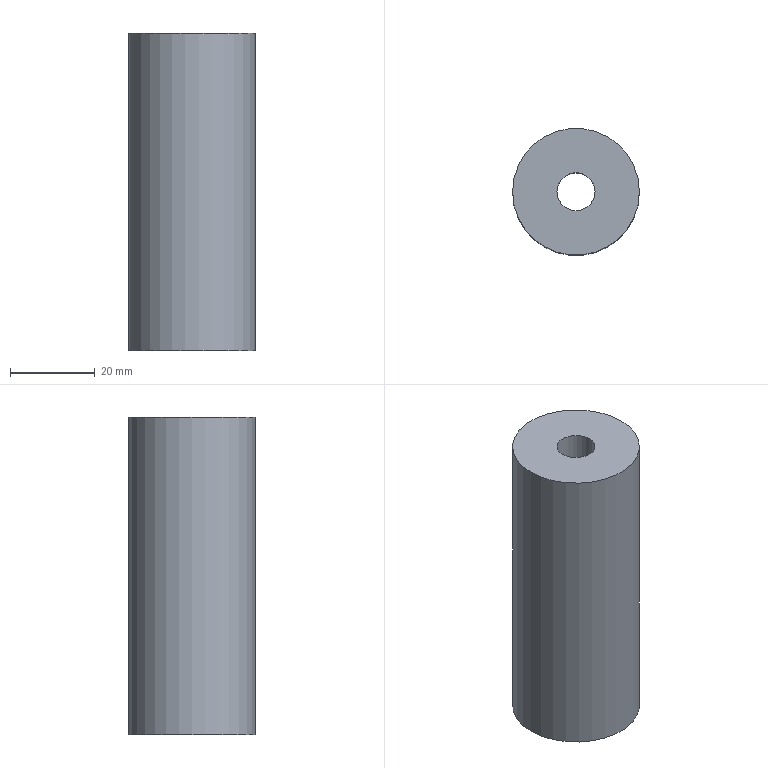Part | NX | features solid 2 | 1 solid | 6 faces | box 30 x 30 x 75 mm | volume 44179 mm3 | cylinder 3 | plane 3 | commonest cylinder face diameters 9 x1 14 x1 30 x1
STEP:
#1=CARTESIAN_POINT('',(-350.023,88.529,-15.002));
#2=VERTEX_POINT('',#1);
#3=CARTESIAN_POINT('',(-335.023,88.529,-15.002));
#4=DIRECTION('',(-0.000000053,0.000000517,-1.));
#5=DIRECTION('',(-1.,0.,0.000000053));
#6=AXIS2_PLACEMENT_3D('',#3,#4,#5);
#7=CIRCLE('',#6,15.);
#8=EDGE_CURVE('',#2,#2,#7,.T.);
#9=ORIENTED_EDGE('',*,*,#8,.F.);
#10=EDGE_LOOP('',(#9));
#11=FACE_BOUND('',#10,.T.);
#12=CARTESIAN_POINT('',(-320.023,88.529,59.998));
#13=VERTEX_POINT('',#12);
#14=CARTESIAN_POINT('',(-335.023,88.529,59.998));
#15=DIRECTION('',(0.000000053,-0.000000517,1.));
#16=DIRECTION('',(1.,0.,-0.000000053));
#17=AXIS2_PLACEMENT_3D('',#14,#15,#16);
#18=CIRCLE('',#17,15.);
#19=EDGE_CURVE('',#13,#13,#18,.F.);
#20=ORIENTED_EDGE('',*,*,#19,.T.);
#21=EDGE_LOOP('',(#20));
#22=FACE_BOUND('',#21,.T.);
#23=CARTESIAN_POINT('',(-335.023,88.529,-24.));
#24=DIRECTION('',(-0.000000053,0.000000517,-1.));
#25=DIRECTION('',(0.,-1.,-0.000000517));
#26=AXIS2_PLACEMENT_3D('',#23,#24,#25);
#27=CYLINDRICAL_SURFACE('',#26,15.);
#28=ADVANCED_FACE('',(#11,#22),#27,.T.);
#29=CARTESIAN_POINT('',(-339.523,88.529,59.998));
#30=VERTEX_POINT('',#29);
#31=CARTESIAN_POINT('',(-335.023,88.529,59.998));
#32=DIRECTION('',(0.000000053,-0.000000517,1.));
#33=DIRECTION('',(-1.,0.,0.000000053));
#34=AXIS2_PLACEMENT_3D('',#31,#32,#33);
#35=CIRCLE('',#34,4.5);
#36=EDGE_CURVE('',#30,#30,#35,.T.);
#37=ORIENTED_EDGE('',*,*,#36,.T.);
#38=EDGE_LOOP('',(#37));
#39=FACE_BOUND('',#38,.T.);
#40=CARTESIAN_POINT('',(-339.523,88.529,29.998));
#41=VERTEX_POINT('',#40);
#42=CARTESIAN_POINT('',(-335.023,88.529,29.998));
#43=DIRECTION('',(0.000000053,-0.000000517,1.));
#44=DIRECTION('',(-1.,0.,0.000000053));
#45=AXIS2_PLACEMENT_3D('',#42,#43,#44);
#46=CIRCLE('',#45,4.5);
#47=EDGE_CURVE('',#41,#41,#46,.T.);
#48=ORIENTED_EDGE('',*,*,#47,.F.);
#49=EDGE_LOOP('',(#48));
#50=FACE_BOUND('',#49,.T.);
#51=CARTESIAN_POINT('',(-335.023,88.529,-64.));
#52=DIRECTION('',(0.000000053,-0.000000517,1.));
#53=DIRECTION('',(0.,-1.,-0.000000517));
#54=AXIS2_PLACEMENT_3D('',#51,#52,#53);
#55=CYLINDRICAL_SURFACE('',#54,4.5);
#56=ADVANCED_FACE('',(#39,#50),#55,.F.);
#57=ORIENTED_EDGE('',*,*,#47,.T.);
#58=EDGE_LOOP('',(#57));
#59=FACE_BOUND('',#58,.T.);
#60=CARTESIAN_POINT('',(-342.023,88.529,29.998));
#61=VERTEX_POINT('',#60);
#62=CARTESIAN_POINT('',(-335.023,88.529,29.998));
#63=DIRECTION('',(0.000000053,-0.000000517,1.));
#64=DIRECTION('',(-1.,0.,0.000000053));
#65=AXIS2_PLACEMENT_3D('',#62,#63,#64);
#66=CIRCLE('',#65,7.);
#67=EDGE_CURVE('',#61,#61,#66,.T.);
#68=ORIENTED_EDGE('',*,*,#67,.F.);
#69=EDGE_LOOP('',(#68));
#70=FACE_BOUND('',#69,.T.);
#71=CARTESIAN_POINT('',(-457.523,261.529,29.998));
#72=DIRECTION('',(-0.000000053,0.000000517,-1.));
#73=DIRECTION('',(1.,0.,-0.000000053));
#74=AXIS2_PLACEMENT_3D('',#71,#72,#73);
#75=PLANE('',#74);
#76=ADVANCED_FACE('',(#59,#70),#75,.T.);
#77=CARTESIAN_POINT('',(-328.023,88.529,-15.002));
#78=VERTEX_POINT('',#77);
#79=CARTESIAN_POINT('',(-335.023,88.529,-15.002));
#80=DIRECTION('',(-0.000000053,0.000000517,-1.));
#81=DIRECTION('',(1.,0.,-0.000000053));
#82=AXIS2_PLACEMENT_3D('',#79,#80,#81);
#83=CIRCLE('',#82,7.);
#84=EDGE_CURVE('',#78,#78,#83,.F.);
#85=ORIENTED_EDGE('',*,*,#84,.F.);
#86=EDGE_LOOP('',(#85));
#87=FACE_BOUND('',#86,.T.);
#88=ORIENTED_EDGE('',*,*,#67,.T.);
#89=EDGE_LOOP('',(#88));
#90=FACE_BOUND('',#89,.T.);
#91=CARTESIAN_POINT('',(-335.023,88.529,-22.));
#92=DIRECTION('',(0.000000053,-0.000000517,1.));
#93=DIRECTION('',(0.,-1.,-0.000000517));
#94=AXIS2_PLACEMENT_3D('',#91,#92,#93);
#95=CYLINDRICAL_SURFACE('',#94,7.);
#96=ADVANCED_FACE('',(#87,#90),#95,.F.);
#97=ORIENTED_EDGE('',*,*,#19,.F.);
#98=EDGE_LOOP('',(#97));
#99=FACE_BOUND('',#98,.T.);
#100=ORIENTED_EDGE('',*,*,#36,.F.);
#101=EDGE_LOOP('',(#100));
#102=FACE_BOUND('',#101,.T.);
#103=CARTESIAN_POINT('',(-335.023,233.529,59.998));
#104=DIRECTION('',(-0.000000053,0.000000517,-1.));
#105=DIRECTION('',(0.,-1.,-0.000000517));
#106=AXIS2_PLACEMENT_3D('',#103,#104,#105);
#107=PLANE('',#106);
#108=ADVANCED_FACE('',(#99,#102),#107,.F.);
#109=ORIENTED_EDGE('',*,*,#8,.T.);
#110=EDGE_LOOP('',(#109));
#111=FACE_BOUND('',#110,.T.);
#112=ORIENTED_EDGE('',*,*,#84,.T.);
#113=EDGE_LOOP('',(#112));
#114=FACE_BOUND('',#113,.T.);
#115=CARTESIAN_POINT('',(-373.023,434.529,-15.001));
#116=DIRECTION('',(0.000000053,-0.000000517,1.));
#117=DIRECTION('',(1.,0.,-0.000000053));
#118=AXIS2_PLACEMENT_3D('',#115,#116,#117);
#119=PLANE('',#118);
#120=ADVANCED_FACE('',(#111,#114),#119,.F.);
#121=CLOSED_SHELL('',(#28,#56,#76,#96,#108,#120));
#122=MANIFOLD_SOLID_BREP('',#121);
#123=(LENGTH_UNIT()NAMED_UNIT(*)SI_UNIT(.MILLI.,.METRE.));
#124=UNCERTAINTY_MEASURE_WITH_UNIT(LENGTH_MEASURE(0.00001),#123,'','');
#125=(NAMED_UNIT(*)PLANE_ANGLE_UNIT()SI_UNIT($,.RADIAN.));
#126=(NAMED_UNIT(*)SI_UNIT($,.STERADIAN.)SOLID_ANGLE_UNIT());
#127=(GEOMETRIC_REPRESENTATION_CONTEXT(3)GLOBAL_UNCERTAINTY_ASSIGNED_CONTEXT((#124))GLOBAL_UNIT_ASSIGNED_CONTEXT((#123,#125,#126))REPRESENTATION_CONTEXT('',''));
#128=ADVANCED_BREP_SHAPE_REPRESENTATION('',(#122),#127);